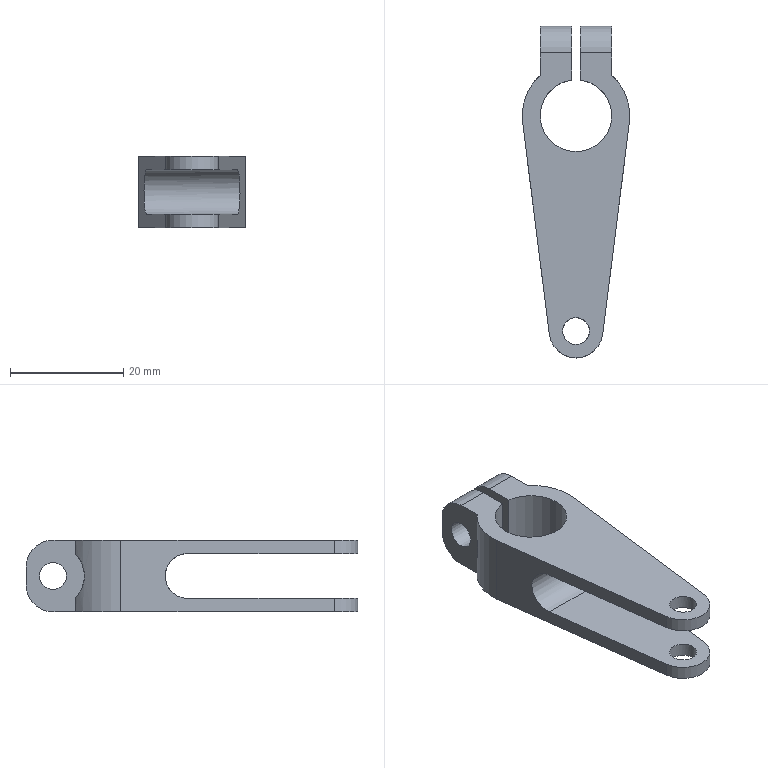Part | NX | features MG0311 small crank arm(0.5 x .190 x 1.5) 2 | 1 solid | 28 faces | box 19.05 x 58.725 x 12.7 mm | volume 4901 mm3 | cylinder 16 | plane 12 | commonest cylinder face diameters 4.763 x4 9.525 x4 9.5 x2 11.113 x2 19.05 x2 7.938 x1
STEP:
#1=CARTESIAN_POINT('',(6.35,7.1,3.843));
#2=VERTEX_POINT('',#1);
#3=CARTESIAN_POINT('',(6.35,7.1,-3.843));
#4=VERTEX_POINT('',#3);
#5=CARTESIAN_POINT('',(6.35,7.1,3.843));
#6=CARTESIAN_POINT('',(6.817,6.682,3.406));
#7=CARTESIAN_POINT('',(7.516,5.884,2.275));
#8=CARTESIAN_POINT('',(7.846,5.393,0.006581));
#9=CARTESIAN_POINT('',(7.518,5.882,-2.273));
#10=CARTESIAN_POINT('',(6.817,6.681,-3.406));
#11=CARTESIAN_POINT('',(6.35,7.1,-3.843));
#12=B_SPLINE_CURVE_WITH_KNOTS('',3,(#5,#6,#7,#8,#9,#10,#11),.UNSPECIFIED.,.F.,.F.,(4,1,1,1,4),(0.,0.002262,0.004524,0.006786,0.009047),.UNSPECIFIED.);
#13=EDGE_CURVE('',#2,#4,#12,.T.);
#14=ORIENTED_EDGE('',*,*,#13,.F.);
#15=CARTESIAN_POINT('',(6.35,7.1,6.35));
#16=VERTEX_POINT('',#15);
#17=CARTESIAN_POINT('',(6.35,7.1,6.35));
#18=DIRECTION('',(0.,0.,-1.));
#19=VECTOR('',#18,1000.);
#20=LINE('',#17,#19);
#21=EDGE_CURVE('',#16,#2,#20,.T.);
#22=ORIENTED_EDGE('',*,*,#21,.F.);
#23=CARTESIAN_POINT('',(9.483,-0.8953,6.35));
#24=VERTEX_POINT('',#23);
#25=CARTESIAN_POINT('',(0.,0.,6.35));
#26=DIRECTION('',(0.,0.,1.));
#27=DIRECTION('',(1.,0.,0.));
#28=AXIS2_PLACEMENT_3D('',#25,#26,#27);
#29=CIRCLE('',#28,9.525);
#30=EDGE_CURVE('',#24,#16,#29,.T.);
#31=ORIENTED_EDGE('',*,*,#30,.F.);
#32=CARTESIAN_POINT('',(9.483,-0.8953,-6.35));
#33=VERTEX_POINT('',#32);
#34=CARTESIAN_POINT('',(9.483,-0.8953,6.35));
#35=DIRECTION('',(0.,0.,-1.));
#36=VECTOR('',#35,1000.);
#37=LINE('',#34,#36);
#38=EDGE_CURVE('',#24,#33,#37,.T.);
#39=ORIENTED_EDGE('',*,*,#38,.T.);
#40=CARTESIAN_POINT('',(6.35,7.1,-6.35));
#41=VERTEX_POINT('',#40);
#42=CARTESIAN_POINT('',(0.,0.,-6.35));
#43=DIRECTION('',(0.,0.,1.));
#44=DIRECTION('',(1.,0.,0.));
#45=AXIS2_PLACEMENT_3D('',#42,#43,#44);
#46=CIRCLE('',#45,9.525);
#47=EDGE_CURVE('',#33,#41,#46,.T.);
#48=ORIENTED_EDGE('',*,*,#47,.T.);
#49=CARTESIAN_POINT('',(6.35,7.1,6.35));
#50=DIRECTION('',(0.,0.,-1.));
#51=VECTOR('',#50,1000.);
#52=LINE('',#49,#51);
#53=EDGE_CURVE('',#4,#41,#52,.T.);
#54=ORIENTED_EDGE('',*,*,#53,.F.);
#55=EDGE_LOOP('',(#14,#22,#31,#39,#48,#54));
#56=FACE_BOUND('',#55,.T.);
#57=CARTESIAN_POINT('',(0.,0.,6.35));
#58=DIRECTION('',(0.,0.,-1.));
#59=DIRECTION('',(-1.,0.,0.));
#60=AXIS2_PLACEMENT_3D('',#57,#58,#59);
#61=CYLINDRICAL_SURFACE('',#60,9.525);
#62=ADVANCED_FACE('',(#56),#61,.T.);
#63=CARTESIAN_POINT('',(-6.35,15.875,1.587));
#64=VERTEX_POINT('',#63);
#65=CARTESIAN_POINT('',(-0.7874,15.875,1.587));
#66=VERTEX_POINT('',#65);
#67=CARTESIAN_POINT('',(6.35,15.875,1.587));
#68=DIRECTION('',(-1.,0.,0.));
#69=VECTOR('',#68,1000.);
#70=LINE('',#67,#69);
#71=EDGE_CURVE('',#64,#66,#70,.F.);
#72=ORIENTED_EDGE('',*,*,#71,.T.);
#73=CARTESIAN_POINT('',(-0.7874,15.875,-1.587));
#74=VERTEX_POINT('',#73);
#75=CARTESIAN_POINT('',(-0.7874,15.875,-6.35));
#76=DIRECTION('',(0.,0.,1.));
#77=VECTOR('',#76,1000.);
#78=LINE('',#75,#77);
#79=EDGE_CURVE('',#74,#66,#78,.T.);
#80=ORIENTED_EDGE('',*,*,#79,.F.);
#81=CARTESIAN_POINT('',(-6.35,15.875,-1.587));
#82=VERTEX_POINT('',#81);
#83=CARTESIAN_POINT('',(-6.35,15.875,-1.587));
#84=DIRECTION('',(-1.,0.,0.));
#85=VECTOR('',#84,1000.);
#86=LINE('',#83,#85);
#87=EDGE_CURVE('',#74,#82,#86,.T.);
#88=ORIENTED_EDGE('',*,*,#87,.T.);
#89=CARTESIAN_POINT('',(-6.35,15.875,6.35));
#90=DIRECTION('',(0.,0.,-1.));
#91=VECTOR('',#90,1000.);
#92=LINE('',#89,#91);
#93=EDGE_CURVE('',#64,#82,#92,.T.);
#94=ORIENTED_EDGE('',*,*,#93,.F.);
#95=EDGE_LOOP('',(#72,#80,#88,#94));
#96=FACE_BOUND('',#95,.T.);
#97=CARTESIAN_POINT('',(-6.35,15.875,6.35));
#98=DIRECTION('',(0.,-1.,0.));
#99=DIRECTION('',(0.,0.,-1.));
#100=AXIS2_PLACEMENT_3D('',#97,#98,#99);
#101=PLANE('',#100);
#102=ADVANCED_FACE('',(#96),#101,.F.);
#103=CARTESIAN_POINT('',(-0.7874,11.113,6.35));
#104=VERTEX_POINT('',#103);
#105=CARTESIAN_POINT('',(-0.7874,11.113,1.587));
#106=DIRECTION('',(-1.,0.,0.));
#107=DIRECTION('',(0.,-1.,0.));
#108=AXIS2_PLACEMENT_3D('',#105,#106,#107);
#109=CIRCLE('',#108,4.763);
#110=EDGE_CURVE('',#66,#104,#109,.F.);
#111=ORIENTED_EDGE('',*,*,#110,.F.);
#112=ORIENTED_EDGE('',*,*,#71,.F.);
#113=CARTESIAN_POINT('',(-6.35,11.113,6.35));
#114=VERTEX_POINT('',#113);
#115=CARTESIAN_POINT('',(-6.35,11.113,1.587));
#116=DIRECTION('',(1.,0.,0.));
#117=DIRECTION('',(0.,1.,0.));
#118=AXIS2_PLACEMENT_3D('',#115,#116,#117);
#119=CIRCLE('',#118,4.763);
#120=EDGE_CURVE('',#114,#64,#119,.F.);
#121=ORIENTED_EDGE('',*,*,#120,.F.);
#122=CARTESIAN_POINT('',(-6.35,11.113,6.35));
#123=DIRECTION('',(-1.,0.,0.));
#124=VECTOR('',#123,1000.);
#125=LINE('',#122,#124);
#126=EDGE_CURVE('',#104,#114,#125,.T.);
#127=ORIENTED_EDGE('',*,*,#126,.F.);
#128=EDGE_LOOP('',(#111,#112,#121,#127));
#129=FACE_BOUND('',#128,.T.);
#130=CARTESIAN_POINT('',(0.,11.113,1.587));
#131=DIRECTION('',(1.,0.,0.));
#132=DIRECTION('',(0.,0.,-1.));
#133=AXIS2_PLACEMENT_3D('',#130,#131,#132);
#134=CYLINDRICAL_SURFACE('',#133,4.763);
#135=ADVANCED_FACE('',(#129),#134,.T.);
#136=CARTESIAN_POINT('',(-0.7874,11.113,-6.35));
#137=VERTEX_POINT('',#136);
#138=CARTESIAN_POINT('',(-0.7874,11.113,-1.587));
#139=DIRECTION('',(-1.,0.,0.));
#140=DIRECTION('',(0.,-1.,0.));
#141=AXIS2_PLACEMENT_3D('',#138,#139,#140);
#142=CIRCLE('',#141,4.763);
#143=EDGE_CURVE('',#137,#74,#142,.F.);
#144=ORIENTED_EDGE('',*,*,#143,.F.);
#145=CARTESIAN_POINT('',(-6.35,11.113,-6.35));
#146=VERTEX_POINT('',#145);
#147=CARTESIAN_POINT('',(0.,11.113,-6.35));
#148=DIRECTION('',(-1.,0.,0.));
#149=VECTOR('',#148,1000.);
#150=LINE('',#147,#149);
#151=EDGE_CURVE('',#146,#137,#150,.F.);
#152=ORIENTED_EDGE('',*,*,#151,.F.);
#153=CARTESIAN_POINT('',(-6.35,11.113,-1.587));
#154=DIRECTION('',(1.,0.,0.));
#155=DIRECTION('',(0.,1.,0.));
#156=AXIS2_PLACEMENT_3D('',#153,#154,#155);
#157=CIRCLE('',#156,4.763);
#158=EDGE_CURVE('',#82,#146,#157,.F.);
#159=ORIENTED_EDGE('',*,*,#158,.F.);
#160=ORIENTED_EDGE('',*,*,#87,.F.);
#161=EDGE_LOOP('',(#144,#152,#159,#160));
#162=FACE_BOUND('',#161,.T.);
#163=CARTESIAN_POINT('',(-6.35,11.113,-1.587));
#164=DIRECTION('',(-1.,0.,0.));
#165=DIRECTION('',(0.,0.,1.));
#166=AXIS2_PLACEMENT_3D('',#163,#164,#165);
#167=CYLINDRICAL_SURFACE('',#166,4.763);
#168=ADVANCED_FACE('',(#162),#167,.T.);
#169=CARTESIAN_POINT('',(-0.7874,8.731,0.));
#170=VERTEX_POINT('',#169);
#171=CARTESIAN_POINT('',(-0.7874,11.113,0.));
#172=DIRECTION('',(-1.,0.,0.));
#173=DIRECTION('',(0.,-1.,0.));
#174=AXIS2_PLACEMENT_3D('',#171,#172,#173);
#175=CIRCLE('',#174,2.381);
#176=EDGE_CURVE('',#170,#170,#175,.F.);
#177=ORIENTED_EDGE('',*,*,#176,.T.);
#178=EDGE_LOOP('',(#177));
#179=FACE_BOUND('',#178,.T.);
#180=CARTESIAN_POINT('',(-6.35,13.494,0.));
#181=VERTEX_POINT('',#180);
#182=CARTESIAN_POINT('',(-6.35,11.113,0.));
#183=DIRECTION('',(1.,0.,0.));
#184=DIRECTION('',(0.,1.,0.));
#185=AXIS2_PLACEMENT_3D('',#182,#183,#184);
#186=CIRCLE('',#185,2.381);
#187=EDGE_CURVE('',#181,#181,#186,.T.);
#188=ORIENTED_EDGE('',*,*,#187,.F.);
#189=EDGE_LOOP('',(#188));
#190=FACE_BOUND('',#189,.T.);
#191=CARTESIAN_POINT('',(-9.525,11.113,0.));
#192=DIRECTION('',(1.,0.,0.));
#193=DIRECTION('',(0.,0.,-1.));
#194=AXIS2_PLACEMENT_3D('',#191,#192,#193);
#195=CYLINDRICAL_SURFACE('',#194,2.381);
#196=ADVANCED_FACE('',(#179,#190),#195,.F.);
#197=CARTESIAN_POINT('',(4.712,-38.695,-3.969));
#198=VERTEX_POINT('',#197);
#199=CARTESIAN_POINT('',(4.712,-38.695,-6.35));
#200=VERTEX_POINT('',#199);
#201=CARTESIAN_POINT('',(4.712,-38.695,6.35));
#202=DIRECTION('',(0.,0.,-1.));
#203=VECTOR('',#202,1000.);
#204=LINE('',#201,#203);
#205=EDGE_CURVE('',#198,#200,#204,.T.);
#206=ORIENTED_EDGE('',*,*,#205,.F.);
#207=CARTESIAN_POINT('',(-4.712,-38.695,-3.969));
#208=VERTEX_POINT('',#207);
#209=CARTESIAN_POINT('',(0.,-38.1,-3.969));
#210=DIRECTION('',(0.,0.,-1.));
#211=DIRECTION('',(0.,1.,0.));
#212=AXIS2_PLACEMENT_3D('',#209,#210,#211);
#213=CIRCLE('',#212,4.75);
#214=EDGE_CURVE('',#198,#208,#213,.T.);
#215=ORIENTED_EDGE('',*,*,#214,.T.);
#216=CARTESIAN_POINT('',(-4.712,-38.695,-6.35));
#217=VERTEX_POINT('',#216);
#218=CARTESIAN_POINT('',(-4.712,-38.695,6.35));
#219=DIRECTION('',(0.,0.,-1.));
#220=VECTOR('',#219,1000.);
#221=LINE('',#218,#220);
#222=EDGE_CURVE('',#208,#217,#221,.T.);
#223=ORIENTED_EDGE('',*,*,#222,.T.);
#224=CARTESIAN_POINT('',(0.,-38.1,-6.35));
#225=DIRECTION('',(0.,0.,1.));
#226=DIRECTION('',(1.,0.,0.));
#227=AXIS2_PLACEMENT_3D('',#224,#225,#226);
#228=CIRCLE('',#227,4.75);
#229=EDGE_CURVE('',#217,#200,#228,.T.);
#230=ORIENTED_EDGE('',*,*,#229,.T.);
#231=EDGE_LOOP('',(#206,#215,#223,#230));
#232=FACE_BOUND('',#231,.T.);
#233=CARTESIAN_POINT('',(0.,-38.1,6.35));
#234=DIRECTION('',(0.,0.,-1.));
#235=DIRECTION('',(-1.,0.,0.));
#236=AXIS2_PLACEMENT_3D('',#233,#234,#235);
#237=CYLINDRICAL_SURFACE('',#236,4.75);
#238=ADVANCED_FACE('',(#232),#237,.T.);
#239=CARTESIAN_POINT('',(0.,-35.719,-3.969));
#240=VERTEX_POINT('',#239);
#241=CARTESIAN_POINT('',(0.,-38.1,-3.969));
#242=DIRECTION('',(0.,0.,-1.));
#243=DIRECTION('',(0.,1.,0.));
#244=AXIS2_PLACEMENT_3D('',#241,#242,#243);
#245=CIRCLE('',#244,2.381);
#246=EDGE_CURVE('',#240,#240,#245,.T.);
#247=ORIENTED_EDGE('',*,*,#246,.F.);
#248=EDGE_LOOP('',(#247));
#249=FACE_BOUND('',#248,.T.);
#250=CARTESIAN_POINT('',(2.381,-38.1,-6.35));
#251=VERTEX_POINT('',#250);
#252=CARTESIAN_POINT('',(0.,-38.1,-6.35));
#253=DIRECTION('',(0.,0.,1.));
#254=DIRECTION('',(1.,0.,0.));
#255=AXIS2_PLACEMENT_3D('',#252,#253,#254);
#256=CIRCLE('',#255,2.381);
#257=EDGE_CURVE('',#251,#251,#256,.T.);
#258=ORIENTED_EDGE('',*,*,#257,.F.);
#259=EDGE_LOOP('',(#258));
#260=FACE_BOUND('',#259,.T.);
#261=CARTESIAN_POINT('',(0.,-38.1,6.35));
#262=DIRECTION('',(0.,0.,-1.));
#263=DIRECTION('',(-1.,0.,0.));
#264=AXIS2_PLACEMENT_3D('',#261,#262,#263);
#265=CYLINDRICAL_SURFACE('',#264,2.381);
#266=ADVANCED_FACE('',(#249,#260),#265,.F.);
#267=CARTESIAN_POINT('',(-0.7874,6.301,6.35));
#268=VERTEX_POINT('',#267);
#269=CARTESIAN_POINT('',(-0.7874,15.875,6.35));
#270=DIRECTION('',(0.,-1.,0.));
#271=VECTOR('',#270,1000.);
#272=LINE('',#269,#271);
#273=EDGE_CURVE('',#104,#268,#272,.T.);
#274=ORIENTED_EDGE('',*,*,#273,.F.);
#275=ORIENTED_EDGE('',*,*,#126,.T.);
#276=CARTESIAN_POINT('',(-6.35,7.1,6.35));
#277=VERTEX_POINT('',#276);
#278=CARTESIAN_POINT('',(-6.35,15.875,6.35));
#279=DIRECTION('',(0.,-1.,0.));
#280=VECTOR('',#279,1000.);
#281=LINE('',#278,#280);
#282=EDGE_CURVE('',#114,#277,#281,.T.);
#283=ORIENTED_EDGE('',*,*,#282,.T.);
#284=CARTESIAN_POINT('',(-9.483,-0.8953,6.35));
#285=VERTEX_POINT('',#284);
#286=CARTESIAN_POINT('',(0.,0.,6.35));
#287=DIRECTION('',(0.,0.,1.));
#288=DIRECTION('',(1.,0.,0.));
#289=AXIS2_PLACEMENT_3D('',#286,#287,#288);
#290=CIRCLE('',#289,9.525);
#291=EDGE_CURVE('',#277,#285,#290,.T.);
#292=ORIENTED_EDGE('',*,*,#291,.T.);
#293=CARTESIAN_POINT('',(-4.712,-38.695,6.35));
#294=VERTEX_POINT('',#293);
#295=CARTESIAN_POINT('',(-9.483,-0.8953,6.35));
#296=DIRECTION('',(0.1252,-0.9921,0.));
#297=VECTOR('',#296,1000.);
#298=LINE('',#295,#297);
#299=EDGE_CURVE('',#285,#294,#298,.T.);
#300=ORIENTED_EDGE('',*,*,#299,.T.);
#301=CARTESIAN_POINT('',(4.712,-38.695,6.35));
#302=VERTEX_POINT('',#301);
#303=CARTESIAN_POINT('',(0.,-38.1,6.35));
#304=DIRECTION('',(0.,0.,1.));
#305=DIRECTION('',(1.,0.,0.));
#306=AXIS2_PLACEMENT_3D('',#303,#304,#305);
#307=CIRCLE('',#306,4.75);
#308=EDGE_CURVE('',#294,#302,#307,.T.);
#309=ORIENTED_EDGE('',*,*,#308,.T.);
#310=CARTESIAN_POINT('',(9.483,-0.8953,6.35));
#311=DIRECTION('',(0.1252,0.9921,0.));
#312=VECTOR('',#311,1000.);
#313=LINE('',#310,#312);
#314=EDGE_CURVE('',#302,#24,#313,.T.);
#315=ORIENTED_EDGE('',*,*,#314,.T.);
#316=ORIENTED_EDGE('',*,*,#30,.T.);
#317=CARTESIAN_POINT('',(6.35,11.113,6.35));
#318=VERTEX_POINT('',#317);
#319=CARTESIAN_POINT('',(6.35,15.875,6.35));
#320=DIRECTION('',(0.,1.,0.));
#321=VECTOR('',#320,1000.);
#322=LINE('',#319,#321);
#323=EDGE_CURVE('',#16,#318,#322,.T.);
#324=ORIENTED_EDGE('',*,*,#323,.T.);
#325=CARTESIAN_POINT('',(0.7874,11.113,6.35));
#326=VERTEX_POINT('',#325);
#327=CARTESIAN_POINT('',(-6.35,11.113,6.35));
#328=DIRECTION('',(-1.,0.,0.));
#329=VECTOR('',#328,1000.);
#330=LINE('',#327,#329);
#331=EDGE_CURVE('',#318,#326,#330,.T.);
#332=ORIENTED_EDGE('',*,*,#331,.T.);
#333=CARTESIAN_POINT('',(0.7874,6.301,6.35));
#334=VERTEX_POINT('',#333);
#335=CARTESIAN_POINT('',(0.7874,15.875,6.35));
#336=DIRECTION('',(0.,1.,0.));
#337=VECTOR('',#336,1000.);
#338=LINE('',#335,#337);
#339=EDGE_CURVE('',#334,#326,#338,.T.);
#340=ORIENTED_EDGE('',*,*,#339,.F.);
#341=CARTESIAN_POINT('',(0.,0.,6.35));
#342=DIRECTION('',(0.,0.,1.));
#343=DIRECTION('',(1.,0.,0.));
#344=AXIS2_PLACEMENT_3D('',#341,#342,#343);
#345=CIRCLE('',#344,6.35);
#346=EDGE_CURVE('',#268,#334,#345,.T.);
#347=ORIENTED_EDGE('',*,*,#346,.F.);
#348=EDGE_LOOP('',(#274,#275,#283,#292,#300,#309,#315,#316,#324,#332,#340,#347));
#349=FACE_BOUND('',#348,.T.);
#350=CARTESIAN_POINT('',(2.381,-38.1,6.35));
#351=VERTEX_POINT('',#350);
#352=CARTESIAN_POINT('',(0.,-38.1,6.35));
#353=DIRECTION('',(0.,0.,1.));
#354=DIRECTION('',(1.,0.,0.));
#355=AXIS2_PLACEMENT_3D('',#352,#353,#354);
#356=CIRCLE('',#355,2.381);
#357=EDGE_CURVE('',#351,#351,#356,.T.);
#358=ORIENTED_EDGE('',*,*,#357,.F.);
#359=EDGE_LOOP('',(#358));
#360=FACE_BOUND('',#359,.T.);
#361=CARTESIAN_POINT('',(0.,0.,6.35));
#362=DIRECTION('',(0.,0.,1.));
#363=DIRECTION('',(1.,0.,0.));
#364=AXIS2_PLACEMENT_3D('',#361,#362,#363);
#365=PLANE('',#364);
#366=ADVANCED_FACE('',(#349,#360),#365,.T.);
#367=ORIENTED_EDGE('',*,*,#151,.T.);
#368=CARTESIAN_POINT('',(-0.7874,6.301,-6.35));
#369=VERTEX_POINT('',#368);
#370=CARTESIAN_POINT('',(-0.7874,15.875,-6.35));
#371=DIRECTION('',(0.,-1.,0.));
#372=VECTOR('',#371,1000.);
#373=LINE('',#370,#372);
#374=EDGE_CURVE('',#137,#369,#373,.T.);
#375=ORIENTED_EDGE('',*,*,#374,.T.);
#376=CARTESIAN_POINT('',(0.7874,6.301,-6.35));
#377=VERTEX_POINT('',#376);
#378=CARTESIAN_POINT('',(0.,0.,-6.35));
#379=DIRECTION('',(0.,0.,1.));
#380=DIRECTION('',(1.,0.,0.));
#381=AXIS2_PLACEMENT_3D('',#378,#379,#380);
#382=CIRCLE('',#381,6.35);
#383=EDGE_CURVE('',#369,#377,#382,.T.);
#384=ORIENTED_EDGE('',*,*,#383,.T.);
#385=CARTESIAN_POINT('',(0.7874,11.113,-6.35));
#386=VERTEX_POINT('',#385);
#387=CARTESIAN_POINT('',(0.7874,15.875,-6.35));
#388=DIRECTION('',(0.,1.,0.));
#389=VECTOR('',#388,1000.);
#390=LINE('',#387,#389);
#391=EDGE_CURVE('',#377,#386,#390,.T.);
#392=ORIENTED_EDGE('',*,*,#391,.T.);
#393=CARTESIAN_POINT('',(6.35,11.113,-6.35));
#394=VERTEX_POINT('',#393);
#395=CARTESIAN_POINT('',(0.,11.113,-6.35));
#396=DIRECTION('',(-1.,0.,0.));
#397=VECTOR('',#396,1000.);
#398=LINE('',#395,#397);
#399=EDGE_CURVE('',#386,#394,#398,.F.);
#400=ORIENTED_EDGE('',*,*,#399,.T.);
#401=CARTESIAN_POINT('',(6.35,15.875,-6.35));
#402=DIRECTION('',(0.,1.,0.));
#403=VECTOR('',#402,1000.);
#404=LINE('',#401,#403);
#405=EDGE_CURVE('',#41,#394,#404,.T.);
#406=ORIENTED_EDGE('',*,*,#405,.F.);
#407=ORIENTED_EDGE('',*,*,#47,.F.);
#408=CARTESIAN_POINT('',(9.483,-0.8953,-6.35));
#409=DIRECTION('',(0.1252,0.9921,0.));
#410=VECTOR('',#409,1000.);
#411=LINE('',#408,#410);
#412=EDGE_CURVE('',#200,#33,#411,.T.);
#413=ORIENTED_EDGE('',*,*,#412,.F.);
#414=ORIENTED_EDGE('',*,*,#229,.F.);
#415=CARTESIAN_POINT('',(-9.483,-0.8953,-6.35));
#416=VERTEX_POINT('',#415);
#417=CARTESIAN_POINT('',(-9.483,-0.8953,-6.35));
#418=DIRECTION('',(0.1252,-0.9921,0.));
#419=VECTOR('',#418,1000.);
#420=LINE('',#417,#419);
#421=EDGE_CURVE('',#416,#217,#420,.T.);
#422=ORIENTED_EDGE('',*,*,#421,.F.);
#423=CARTESIAN_POINT('',(-6.35,7.1,-6.35));
#424=VERTEX_POINT('',#423);
#425=CARTESIAN_POINT('',(0.,0.,-6.35));
#426=DIRECTION('',(0.,0.,1.));
#427=DIRECTION('',(1.,0.,0.));
#428=AXIS2_PLACEMENT_3D('',#425,#426,#427);
#429=CIRCLE('',#428,9.525);
#430=EDGE_CURVE('',#424,#416,#429,.T.);
#431=ORIENTED_EDGE('',*,*,#430,.F.);
#432=CARTESIAN_POINT('',(-6.35,15.875,-6.35));
#433=DIRECTION('',(0.,-1.,0.));
#434=VECTOR('',#433,1000.);
#435=LINE('',#432,#434);
#436=EDGE_CURVE('',#146,#424,#435,.T.);
#437=ORIENTED_EDGE('',*,*,#436,.F.);
#438=EDGE_LOOP('',(#367,#375,#384,#392,#400,#406,#407,#413,#414,#422,#431,#437));
#439=FACE_BOUND('',#438,.T.);
#440=ORIENTED_EDGE('',*,*,#257,.T.);
#441=EDGE_LOOP('',(#440));
#442=FACE_BOUND('',#441,.T.);
#443=CARTESIAN_POINT('',(0.,0.,-6.35));
#444=DIRECTION('',(0.,0.,1.));
#445=DIRECTION('',(1.,0.,0.));
#446=AXIS2_PLACEMENT_3D('',#443,#444,#445);
#447=PLANE('',#446);
#448=ADVANCED_FACE('',(#439,#442),#447,.F.);
#449=CARTESIAN_POINT('',(-6.35,7.1,-3.843));
#450=VERTEX_POINT('',#449);
#451=CARTESIAN_POINT('',(-6.35,7.1,6.35));
#452=DIRECTION('',(0.,0.,-1.));
#453=VECTOR('',#452,1000.);
#454=LINE('',#451,#453);
#455=EDGE_CURVE('',#450,#424,#454,.T.);
#456=ORIENTED_EDGE('',*,*,#455,.F.);
#457=CARTESIAN_POINT('',(-6.35,7.1,3.843));
#458=VERTEX_POINT('',#457);
#459=CARTESIAN_POINT('',(-6.35,11.113,0.));
#460=DIRECTION('',(1.,0.,0.));
#461=DIRECTION('',(0.,0.,-1.));
#462=AXIS2_PLACEMENT_3D('',#459,#460,#461);
#463=CIRCLE('',#462,5.556);
#464=EDGE_CURVE('',#458,#450,#463,.T.);
#465=ORIENTED_EDGE('',*,*,#464,.F.);
#466=CARTESIAN_POINT('',(-6.35,7.1,6.35));
#467=DIRECTION('',(0.,0.,-1.));
#468=VECTOR('',#467,1000.);
#469=LINE('',#466,#468);
#470=EDGE_CURVE('',#277,#458,#469,.T.);
#471=ORIENTED_EDGE('',*,*,#470,.F.);
#472=ORIENTED_EDGE('',*,*,#282,.F.);
#473=ORIENTED_EDGE('',*,*,#120,.T.);
#474=ORIENTED_EDGE('',*,*,#93,.T.);
#475=ORIENTED_EDGE('',*,*,#158,.T.);
#476=ORIENTED_EDGE('',*,*,#436,.T.);
#477=EDGE_LOOP('',(#456,#465,#471,#472,#473,#474,#475,#476));
#478=FACE_BOUND('',#477,.T.);
#479=ORIENTED_EDGE('',*,*,#187,.T.);
#480=EDGE_LOOP('',(#479));
#481=FACE_BOUND('',#480,.T.);
#482=CARTESIAN_POINT('',(-6.35,15.875,6.35));
#483=DIRECTION('',(1.,0.,0.));
#484=DIRECTION('',(0.,1.,0.));
#485=AXIS2_PLACEMENT_3D('',#482,#483,#484);
#486=PLANE('',#485);
#487=ADVANCED_FACE('',(#478,#481),#486,.F.);
#488=ORIENTED_EDGE('',*,*,#470,.T.);
#489=CARTESIAN_POINT('',(-6.35,7.1,3.843));
#490=CARTESIAN_POINT('',(-6.817,6.682,3.406));
#491=CARTESIAN_POINT('',(-7.516,5.884,2.275));
#492=CARTESIAN_POINT('',(-7.846,5.393,0.006581));
#493=CARTESIAN_POINT('',(-7.518,5.882,-2.273));
#494=CARTESIAN_POINT('',(-6.817,6.681,-3.406));
#495=CARTESIAN_POINT('',(-6.35,7.1,-3.843));
#496=B_SPLINE_CURVE_WITH_KNOTS('',3,(#489,#490,#491,#492,#493,#494,#495),.UNSPECIFIED.,.F.,.F.,(4,1,1,1,4),(0.,0.002262,0.004524,0.006786,0.009047),.UNSPECIFIED.);
#497=EDGE_CURVE('',#458,#450,#496,.T.);
#498=ORIENTED_EDGE('',*,*,#497,.T.);
#499=ORIENTED_EDGE('',*,*,#455,.T.);
#500=ORIENTED_EDGE('',*,*,#430,.T.);
#501=CARTESIAN_POINT('',(-9.483,-0.8953,6.35));
#502=DIRECTION('',(0.,0.,-1.));
#503=VECTOR('',#502,1000.);
#504=LINE('',#501,#503);
#505=EDGE_CURVE('',#285,#416,#504,.T.);
#506=ORIENTED_EDGE('',*,*,#505,.F.);
#507=ORIENTED_EDGE('',*,*,#291,.F.);
#508=EDGE_LOOP('',(#488,#498,#499,#500,#506,#507));
#509=FACE_BOUND('',#508,.T.);
#510=CARTESIAN_POINT('',(0.,0.,6.35));
#511=DIRECTION('',(0.,0.,-1.));
#512=DIRECTION('',(-1.,0.,0.));
#513=AXIS2_PLACEMENT_3D('',#510,#511,#512);
#514=CYLINDRICAL_SURFACE('',#513,9.525);
#515=ADVANCED_FACE('',(#509),#514,.T.);
#516=ORIENTED_EDGE('',*,*,#222,.F.);
#517=CARTESIAN_POINT('',(-7.993,-12.7,-3.969));
#518=VERTEX_POINT('',#517);
#519=CARTESIAN_POINT('',(-9.483,-0.8953,-3.969));
#520=DIRECTION('',(-0.1252,0.9921,0.));
#521=VECTOR('',#520,1000.);
#522=LINE('',#519,#521);
#523=EDGE_CURVE('',#208,#518,#522,.T.);
#524=ORIENTED_EDGE('',*,*,#523,.T.);
#525=CARTESIAN_POINT('',(-7.993,-12.7,3.969));
#526=VERTEX_POINT('',#525);
#527=CARTESIAN_POINT('',(-7.993,-12.7,0.));
#528=DIRECTION('',(0.9921,0.1252,0.));
#529=DIRECTION('',(0.1252,-0.9921,0.));
#530=AXIS2_PLACEMENT_3D('',#527,#528,#529);
#531=ELLIPSE('',#530,4.,3.969);
#532=EDGE_CURVE('',#518,#526,#531,.T.);
#533=ORIENTED_EDGE('',*,*,#532,.T.);
#534=CARTESIAN_POINT('',(-4.712,-38.695,3.969));
#535=VERTEX_POINT('',#534);
#536=CARTESIAN_POINT('',(-9.483,-0.8953,3.969));
#537=DIRECTION('',(0.1252,-0.9921,0.));
#538=VECTOR('',#537,1000.);
#539=LINE('',#536,#538);
#540=EDGE_CURVE('',#526,#535,#539,.T.);
#541=ORIENTED_EDGE('',*,*,#540,.T.);
#542=CARTESIAN_POINT('',(-4.712,-38.695,6.35));
#543=DIRECTION('',(0.,0.,-1.));
#544=VECTOR('',#543,1000.);
#545=LINE('',#542,#544);
#546=EDGE_CURVE('',#294,#535,#545,.T.);
#547=ORIENTED_EDGE('',*,*,#546,.F.);
#548=ORIENTED_EDGE('',*,*,#299,.F.);
#549=ORIENTED_EDGE('',*,*,#505,.T.);
#550=ORIENTED_EDGE('',*,*,#421,.T.);
#551=EDGE_LOOP('',(#516,#524,#533,#541,#547,#548,#549,#550));
#552=FACE_BOUND('',#551,.T.);
#553=CARTESIAN_POINT('',(-9.483,-0.8953,6.35));
#554=DIRECTION('',(0.9921,0.1252,0.));
#555=DIRECTION('',(-0.1252,0.9921,0.));
#556=AXIS2_PLACEMENT_3D('',#553,#554,#555);
#557=PLANE('',#556);
#558=ADVANCED_FACE('',(#552),#557,.F.);
#559=CARTESIAN_POINT('',(4.712,-38.695,3.969));
#560=VERTEX_POINT('',#559);
#561=CARTESIAN_POINT('',(0.,-38.1,3.969));
#562=DIRECTION('',(0.,0.,1.));
#563=DIRECTION('',(0.,-1.,0.));
#564=AXIS2_PLACEMENT_3D('',#561,#562,#563);
#565=CIRCLE('',#564,4.75);
#566=EDGE_CURVE('',#535,#560,#565,.T.);
#567=ORIENTED_EDGE('',*,*,#566,.T.);
#568=CARTESIAN_POINT('',(4.712,-38.695,6.35));
#569=DIRECTION('',(0.,0.,-1.));
#570=VECTOR('',#569,1000.);
#571=LINE('',#568,#570);
#572=EDGE_CURVE('',#302,#560,#571,.T.);
#573=ORIENTED_EDGE('',*,*,#572,.F.);
#574=ORIENTED_EDGE('',*,*,#308,.F.);
#575=ORIENTED_EDGE('',*,*,#546,.T.);
#576=EDGE_LOOP('',(#567,#573,#574,#575));
#577=FACE_BOUND('',#576,.T.);
#578=CARTESIAN_POINT('',(0.,-38.1,6.35));
#579=DIRECTION('',(0.,0.,-1.));
#580=DIRECTION('',(-1.,0.,0.));
#581=AXIS2_PLACEMENT_3D('',#578,#579,#580);
#582=CYLINDRICAL_SURFACE('',#581,4.75);
#583=ADVANCED_FACE('',(#577),#582,.T.);
#584=CARTESIAN_POINT('',(7.993,-12.7,3.969));
#585=VERTEX_POINT('',#584);
#586=CARTESIAN_POINT('',(7.993,-12.7,-3.969));
#587=VERTEX_POINT('',#586);
#588=CARTESIAN_POINT('',(7.993,-12.7,0.));
#589=DIRECTION('',(-0.9921,0.1252,0.));
#590=DIRECTION('',(0.1252,0.9921,0.));
#591=AXIS2_PLACEMENT_3D('',#588,#589,#590);
#592=ELLIPSE('',#591,4.,3.969);
#593=EDGE_CURVE('',#585,#587,#592,.T.);
#594=ORIENTED_EDGE('',*,*,#593,.T.);
#595=CARTESIAN_POINT('',(9.483,-0.8953,-3.969));
#596=DIRECTION('',(-0.1252,-0.9921,0.));
#597=VECTOR('',#596,1000.);
#598=LINE('',#595,#597);
#599=EDGE_CURVE('',#587,#198,#598,.T.);
#600=ORIENTED_EDGE('',*,*,#599,.T.);
#601=ORIENTED_EDGE('',*,*,#205,.T.);
#602=ORIENTED_EDGE('',*,*,#412,.T.);
#603=ORIENTED_EDGE('',*,*,#38,.F.);
#604=ORIENTED_EDGE('',*,*,#314,.F.);
#605=ORIENTED_EDGE('',*,*,#572,.T.);
#606=CARTESIAN_POINT('',(9.483,-0.8953,3.969));
#607=DIRECTION('',(0.1252,0.9921,0.));
#608=VECTOR('',#607,1000.);
#609=LINE('',#606,#608);
#610=EDGE_CURVE('',#560,#585,#609,.T.);
#611=ORIENTED_EDGE('',*,*,#610,.T.);
#612=EDGE_LOOP('',(#594,#600,#601,#602,#603,#604,#605,#611));
#613=FACE_BOUND('',#612,.T.);
#614=CARTESIAN_POINT('',(9.483,-0.8953,6.35));
#615=DIRECTION('',(-0.9921,0.1252,0.));
#616=DIRECTION('',(-0.1252,-0.9921,0.));
#617=AXIS2_PLACEMENT_3D('',#614,#615,#616);
#618=PLANE('',#617);
#619=ADVANCED_FACE('',(#613),#618,.F.);
#620=ORIENTED_EDGE('',*,*,#21,.T.);
#621=CARTESIAN_POINT('',(6.35,11.113,0.));
#622=DIRECTION('',(1.,0.,0.));
#623=DIRECTION('',(0.,0.,-1.));
#624=AXIS2_PLACEMENT_3D('',#621,#622,#623);
#625=CIRCLE('',#624,5.556);
#626=EDGE_CURVE('',#2,#4,#625,.T.);
#627=ORIENTED_EDGE('',*,*,#626,.T.);
#628=ORIENTED_EDGE('',*,*,#53,.T.);
#629=ORIENTED_EDGE('',*,*,#405,.T.);
#630=CARTESIAN_POINT('',(6.35,15.875,-1.587));
#631=VERTEX_POINT('',#630);
#632=CARTESIAN_POINT('',(6.35,11.113,-1.587));
#633=DIRECTION('',(-1.,0.,0.));
#634=DIRECTION('',(0.,-1.,0.));
#635=AXIS2_PLACEMENT_3D('',#632,#633,#634);
#636=CIRCLE('',#635,4.763);
#637=EDGE_CURVE('',#394,#631,#636,.F.);
#638=ORIENTED_EDGE('',*,*,#637,.T.);
#639=CARTESIAN_POINT('',(6.35,15.875,1.587));
#640=VERTEX_POINT('',#639);
#641=CARTESIAN_POINT('',(6.35,15.875,6.35));
#642=DIRECTION('',(0.,0.,-1.));
#643=VECTOR('',#642,1000.);
#644=LINE('',#641,#643);
#645=EDGE_CURVE('',#640,#631,#644,.T.);
#646=ORIENTED_EDGE('',*,*,#645,.F.);
#647=CARTESIAN_POINT('',(6.35,11.113,1.587));
#648=DIRECTION('',(-1.,0.,0.));
#649=DIRECTION('',(0.,-1.,0.));
#650=AXIS2_PLACEMENT_3D('',#647,#648,#649);
#651=CIRCLE('',#650,4.763);
#652=EDGE_CURVE('',#640,#318,#651,.F.);
#653=ORIENTED_EDGE('',*,*,#652,.T.);
#654=ORIENTED_EDGE('',*,*,#323,.F.);
#655=EDGE_LOOP('',(#620,#627,#628,#629,#638,#646,#653,#654));
#656=FACE_BOUND('',#655,.T.);
#657=CARTESIAN_POINT('',(6.35,8.731,0.));
#658=VERTEX_POINT('',#657);
#659=CARTESIAN_POINT('',(6.35,11.113,0.));
#660=DIRECTION('',(-1.,0.,0.));
#661=DIRECTION('',(0.,-1.,0.));
#662=AXIS2_PLACEMENT_3D('',#659,#660,#661);
#663=CIRCLE('',#662,2.381);
#664=EDGE_CURVE('',#658,#658,#663,.T.);
#665=ORIENTED_EDGE('',*,*,#664,.T.);
#666=EDGE_LOOP('',(#665));
#667=FACE_BOUND('',#666,.T.);
#668=CARTESIAN_POINT('',(6.35,15.875,6.35));
#669=DIRECTION('',(-1.,0.,0.));
#670=DIRECTION('',(0.,-1.,0.));
#671=AXIS2_PLACEMENT_3D('',#668,#669,#670);
#672=PLANE('',#671);
#673=ADVANCED_FACE('',(#656,#667),#672,.F.);
#674=CARTESIAN_POINT('',(0.7874,15.875,-1.587));
#675=VERTEX_POINT('',#674);
#676=CARTESIAN_POINT('',(-6.35,15.875,-1.587));
#677=DIRECTION('',(-1.,0.,0.));
#678=VECTOR('',#677,1000.);
#679=LINE('',#676,#678);
#680=EDGE_CURVE('',#631,#675,#679,.T.);
#681=ORIENTED_EDGE('',*,*,#680,.T.);
#682=CARTESIAN_POINT('',(0.7874,15.875,1.587));
#683=VERTEX_POINT('',#682);
#684=CARTESIAN_POINT('',(0.7874,15.875,-6.35));
#685=DIRECTION('',(0.,0.,1.));
#686=VECTOR('',#685,1000.);
#687=LINE('',#684,#686);
#688=EDGE_CURVE('',#675,#683,#687,.T.);
#689=ORIENTED_EDGE('',*,*,#688,.T.);
#690=CARTESIAN_POINT('',(6.35,15.875,1.587));
#691=DIRECTION('',(-1.,0.,0.));
#692=VECTOR('',#691,1000.);
#693=LINE('',#690,#692);
#694=EDGE_CURVE('',#683,#640,#693,.F.);
#695=ORIENTED_EDGE('',*,*,#694,.T.);
#696=ORIENTED_EDGE('',*,*,#645,.T.);
#697=EDGE_LOOP('',(#681,#689,#695,#696));
#698=FACE_BOUND('',#697,.T.);
#699=CARTESIAN_POINT('',(-6.35,15.875,6.35));
#700=DIRECTION('',(0.,-1.,0.));
#701=DIRECTION('',(0.,0.,-1.));
#702=AXIS2_PLACEMENT_3D('',#699,#700,#701);
#703=PLANE('',#702);
#704=ADVANCED_FACE('',(#698),#703,.F.);
#705=CARTESIAN_POINT('',(-0.7874,6.301,6.35));
#706=DIRECTION('',(0.,0.,-1.));
#707=VECTOR('',#706,1000.);
#708=LINE('',#705,#707);
#709=EDGE_CURVE('',#268,#369,#708,.T.);
#710=ORIENTED_EDGE('',*,*,#709,.F.);
#711=ORIENTED_EDGE('',*,*,#346,.T.);
#712=CARTESIAN_POINT('',(0.7874,6.301,6.35));
#713=DIRECTION('',(0.,0.,-1.));
#714=VECTOR('',#713,1000.);
#715=LINE('',#712,#714);
#716=EDGE_CURVE('',#377,#334,#715,.F.);
#717=ORIENTED_EDGE('',*,*,#716,.F.);
#718=ORIENTED_EDGE('',*,*,#383,.F.);
#719=EDGE_LOOP('',(#710,#711,#717,#718));
#720=FACE_BOUND('',#719,.T.);
#721=CARTESIAN_POINT('',(0.,0.,6.35));
#722=DIRECTION('',(0.,0.,-1.));
#723=DIRECTION('',(-1.,0.,0.));
#724=AXIS2_PLACEMENT_3D('',#721,#722,#723);
#725=CYLINDRICAL_SURFACE('',#724,6.35);
#726=ADVANCED_FACE('',(#720),#725,.F.);
#727=CARTESIAN_POINT('',(0.,-40.481,3.969));
#728=VERTEX_POINT('',#727);
#729=CARTESIAN_POINT('',(0.,-38.1,3.969));
#730=DIRECTION('',(0.,0.,1.));
#731=DIRECTION('',(0.,-1.,0.));
#732=AXIS2_PLACEMENT_3D('',#729,#730,#731);
#733=CIRCLE('',#732,2.381);
#734=EDGE_CURVE('',#728,#728,#733,.T.);
#735=ORIENTED_EDGE('',*,*,#734,.F.);
#736=EDGE_LOOP('',(#735));
#737=FACE_BOUND('',#736,.T.);
#738=ORIENTED_EDGE('',*,*,#357,.T.);
#739=EDGE_LOOP('',(#738));
#740=FACE_BOUND('',#739,.T.);
#741=CARTESIAN_POINT('',(0.,-38.1,6.35));
#742=DIRECTION('',(0.,0.,-1.));
#743=DIRECTION('',(-1.,0.,0.));
#744=AXIS2_PLACEMENT_3D('',#741,#742,#743);
#745=CYLINDRICAL_SURFACE('',#744,2.381);
#746=ADVANCED_FACE('',(#737,#740),#745,.F.);
#747=CARTESIAN_POINT('',(0.7874,11.113,1.587));
#748=DIRECTION('',(1.,0.,0.));
#749=DIRECTION('',(0.,1.,0.));
#750=AXIS2_PLACEMENT_3D('',#747,#748,#749);
#751=CIRCLE('',#750,4.763);
#752=EDGE_CURVE('',#326,#683,#751,.F.);
#753=ORIENTED_EDGE('',*,*,#752,.F.);
#754=ORIENTED_EDGE('',*,*,#331,.F.);
#755=ORIENTED_EDGE('',*,*,#652,.F.);
#756=ORIENTED_EDGE('',*,*,#694,.F.);
#757=EDGE_LOOP('',(#753,#754,#755,#756));
#758=FACE_BOUND('',#757,.T.);
#759=CARTESIAN_POINT('',(0.,11.113,1.587));
#760=DIRECTION('',(1.,0.,0.));
#761=DIRECTION('',(0.,0.,-1.));
#762=AXIS2_PLACEMENT_3D('',#759,#760,#761);
#763=CYLINDRICAL_SURFACE('',#762,4.763);
#764=ADVANCED_FACE('',(#758),#763,.T.);
#765=CARTESIAN_POINT('',(0.7874,11.113,-1.587));
#766=DIRECTION('',(1.,0.,0.));
#767=DIRECTION('',(0.,1.,0.));
#768=AXIS2_PLACEMENT_3D('',#765,#766,#767);
#769=CIRCLE('',#768,4.763);
#770=EDGE_CURVE('',#675,#386,#769,.F.);
#771=ORIENTED_EDGE('',*,*,#770,.F.);
#772=ORIENTED_EDGE('',*,*,#680,.F.);
#773=ORIENTED_EDGE('',*,*,#637,.F.);
#774=ORIENTED_EDGE('',*,*,#399,.F.);
#775=EDGE_LOOP('',(#771,#772,#773,#774));
#776=FACE_BOUND('',#775,.T.);
#777=CARTESIAN_POINT('',(-6.35,11.113,-1.587));
#778=DIRECTION('',(-1.,0.,0.));
#779=DIRECTION('',(0.,0.,1.));
#780=AXIS2_PLACEMENT_3D('',#777,#778,#779);
#781=CYLINDRICAL_SURFACE('',#780,4.763);
#782=ADVANCED_FACE('',(#776),#781,.T.);
#783=CARTESIAN_POINT('',(-9.525,-12.7,-3.969));
#784=DIRECTION('',(1.,0.,0.));
#785=VECTOR('',#784,1000.);
#786=LINE('',#783,#785);
#787=EDGE_CURVE('',#518,#587,#786,.T.);
#788=ORIENTED_EDGE('',*,*,#787,.T.);
#789=ORIENTED_EDGE('',*,*,#593,.F.);
#790=CARTESIAN_POINT('',(-9.525,-12.7,3.969));
#791=DIRECTION('',(1.,0.,0.));
#792=VECTOR('',#791,1000.);
#793=LINE('',#790,#792);
#794=EDGE_CURVE('',#526,#585,#793,.T.);
#795=ORIENTED_EDGE('',*,*,#794,.F.);
#796=ORIENTED_EDGE('',*,*,#532,.F.);
#797=EDGE_LOOP('',(#788,#789,#795,#796));
#798=FACE_BOUND('',#797,.T.);
#799=CARTESIAN_POINT('',(-9.525,-12.7,0.));
#800=DIRECTION('',(1.,0.,0.));
#801=DIRECTION('',(0.,0.,-1.));
#802=AXIS2_PLACEMENT_3D('',#799,#800,#801);
#803=CYLINDRICAL_SURFACE('',#802,3.969);
#804=ADVANCED_FACE('',(#798),#803,.F.);
#805=ORIENTED_EDGE('',*,*,#246,.T.);
#806=EDGE_LOOP('',(#805));
#807=FACE_BOUND('',#806,.T.);
#808=ORIENTED_EDGE('',*,*,#214,.F.);
#809=ORIENTED_EDGE('',*,*,#599,.F.);
#810=ORIENTED_EDGE('',*,*,#787,.F.);
#811=ORIENTED_EDGE('',*,*,#523,.F.);
#812=EDGE_LOOP('',(#808,#809,#810,#811));
#813=FACE_BOUND('',#812,.T.);
#814=CARTESIAN_POINT('',(-9.525,-12.7,-3.969));
#815=DIRECTION('',(0.,0.,-1.));
#816=DIRECTION('',(0.,1.,0.));
#817=AXIS2_PLACEMENT_3D('',#814,#815,#816);
#818=PLANE('',#817);
#819=ADVANCED_FACE('',(#807,#813),#818,.F.);
#820=ORIENTED_EDGE('',*,*,#734,.T.);
#821=EDGE_LOOP('',(#820));
#822=FACE_BOUND('',#821,.T.);
#823=ORIENTED_EDGE('',*,*,#794,.T.);
#824=ORIENTED_EDGE('',*,*,#610,.F.);
#825=ORIENTED_EDGE('',*,*,#566,.F.);
#826=ORIENTED_EDGE('',*,*,#540,.F.);
#827=EDGE_LOOP('',(#823,#824,#825,#826));
#828=FACE_BOUND('',#827,.T.);
#829=CARTESIAN_POINT('',(-9.525,-12.7,3.969));
#830=DIRECTION('',(0.,0.,1.));
#831=DIRECTION('',(0.,-1.,0.));
#832=AXIS2_PLACEMENT_3D('',#829,#830,#831);
#833=PLANE('',#832);
#834=ADVANCED_FACE('',(#822,#828),#833,.F.);
#835=CARTESIAN_POINT('',(0.7874,13.494,0.));
#836=VERTEX_POINT('',#835);
#837=CARTESIAN_POINT('',(0.7874,11.113,0.));
#838=DIRECTION('',(1.,0.,0.));
#839=DIRECTION('',(0.,1.,0.));
#840=AXIS2_PLACEMENT_3D('',#837,#838,#839);
#841=CIRCLE('',#840,2.381);
#842=EDGE_CURVE('',#836,#836,#841,.F.);
#843=ORIENTED_EDGE('',*,*,#842,.T.);
#844=EDGE_LOOP('',(#843));
#845=FACE_BOUND('',#844,.T.);
#846=ORIENTED_EDGE('',*,*,#664,.F.);
#847=EDGE_LOOP('',(#846));
#848=FACE_BOUND('',#847,.T.);
#849=CARTESIAN_POINT('',(-9.525,11.113,0.));
#850=DIRECTION('',(1.,0.,0.));
#851=DIRECTION('',(0.,0.,-1.));
#852=AXIS2_PLACEMENT_3D('',#849,#850,#851);
#853=CYLINDRICAL_SURFACE('',#852,2.381);
#854=ADVANCED_FACE('',(#845,#848),#853,.F.);
#855=ORIENTED_EDGE('',*,*,#716,.T.);
#856=ORIENTED_EDGE('',*,*,#339,.T.);
#857=ORIENTED_EDGE('',*,*,#752,.T.);
#858=ORIENTED_EDGE('',*,*,#688,.F.);
#859=ORIENTED_EDGE('',*,*,#770,.T.);
#860=ORIENTED_EDGE('',*,*,#391,.F.);
#861=EDGE_LOOP('',(#855,#856,#857,#858,#859,#860));
#862=FACE_BOUND('',#861,.T.);
#863=ORIENTED_EDGE('',*,*,#842,.F.);
#864=EDGE_LOOP('',(#863));
#865=FACE_BOUND('',#864,.T.);
#866=CARTESIAN_POINT('',(0.7874,15.875,-6.35));
#867=DIRECTION('',(1.,0.,0.));
#868=DIRECTION('',(0.,1.,0.));
#869=AXIS2_PLACEMENT_3D('',#866,#867,#868);
#870=PLANE('',#869);
#871=ADVANCED_FACE('',(#862,#865),#870,.F.);
#872=ORIENTED_EDGE('',*,*,#709,.T.);
#873=ORIENTED_EDGE('',*,*,#374,.F.);
#874=ORIENTED_EDGE('',*,*,#143,.T.);
#875=ORIENTED_EDGE('',*,*,#79,.T.);
#876=ORIENTED_EDGE('',*,*,#110,.T.);
#877=ORIENTED_EDGE('',*,*,#273,.T.);
#878=EDGE_LOOP('',(#872,#873,#874,#875,#876,#877));
#879=FACE_BOUND('',#878,.T.);
#880=ORIENTED_EDGE('',*,*,#176,.F.);
#881=EDGE_LOOP('',(#880));
#882=FACE_BOUND('',#881,.T.);
#883=CARTESIAN_POINT('',(-0.7874,15.875,-6.35));
#884=DIRECTION('',(-1.,0.,0.));
#885=DIRECTION('',(0.,-1.,0.));
#886=AXIS2_PLACEMENT_3D('',#883,#884,#885);
#887=PLANE('',#886);
#888=ADVANCED_FACE('',(#879,#882),#887,.F.);
#889=ORIENTED_EDGE('',*,*,#13,.T.);
#890=ORIENTED_EDGE('',*,*,#626,.F.);
#891=EDGE_LOOP('',(#889,#890));
#892=FACE_BOUND('',#891,.T.);
#893=CARTESIAN_POINT('',(9.525,11.113,0.));
#894=DIRECTION('',(-1.,0.,0.));
#895=DIRECTION('',(0.,0.,1.));
#896=AXIS2_PLACEMENT_3D('',#893,#894,#895);
#897=CYLINDRICAL_SURFACE('',#896,5.556);
#898=ADVANCED_FACE('',(#892),#897,.F.);
#899=ORIENTED_EDGE('',*,*,#464,.T.);
#900=ORIENTED_EDGE('',*,*,#497,.F.);
#901=EDGE_LOOP('',(#899,#900));
#902=FACE_BOUND('',#901,.T.);
#903=CARTESIAN_POINT('',(-9.525,11.113,0.));
#904=DIRECTION('',(1.,0.,0.));
#905=DIRECTION('',(0.,0.,-1.));
#906=AXIS2_PLACEMENT_3D('',#903,#904,#905);
#907=CYLINDRICAL_SURFACE('',#906,5.556);
#908=ADVANCED_FACE('',(#902),#907,.F.);
#909=CLOSED_SHELL('',(#62,#102,#135,#168,#196,#238,#266,#366,#448,#487,#515,#558,#583,#619,#673,#704,#726,#746,#764,#782,#804,#819,#834,#854,#871,#888,#898,#908));
#910=MANIFOLD_SOLID_BREP('',#909);
#911=(LENGTH_UNIT()NAMED_UNIT(*)SI_UNIT(.MILLI.,.METRE.));
#912=UNCERTAINTY_MEASURE_WITH_UNIT(LENGTH_MEASURE(0.0508),#911,'','');
#913=(NAMED_UNIT(*)PLANE_ANGLE_UNIT()SI_UNIT($,.RADIAN.));
#914=(NAMED_UNIT(*)SI_UNIT($,.STERADIAN.)SOLID_ANGLE_UNIT());
#915=(GEOMETRIC_REPRESENTATION_CONTEXT(3)GLOBAL_UNCERTAINTY_ASSIGNED_CONTEXT((#912))GLOBAL_UNIT_ASSIGNED_CONTEXT((#911,#913,#914))REPRESENTATION_CONTEXT('',''));
#916=ADVANCED_BREP_SHAPE_REPRESENTATION('',(#910),#915);